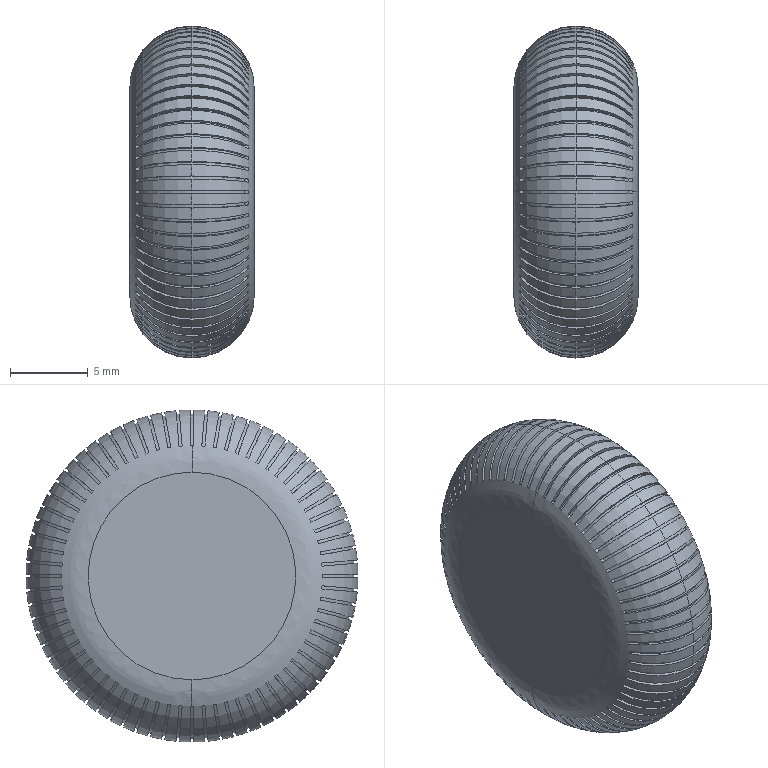Part | STEP file | Guide wheel mechanism revised.sldasm-Part-310 | 1 solid | 366 faces | box 8 x 21.346 x 21.346 mm | volume 2417 mm3 | plane 290 | cylinder 72 | spline 4 | commonest cylinder face diameters 7.6 x72